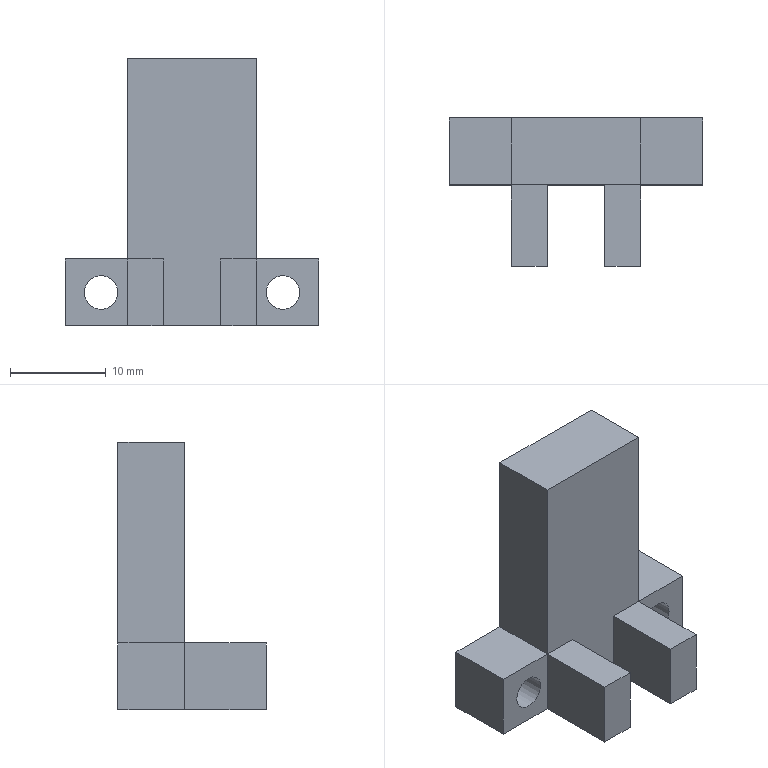Part | NX | 1 solid | 22 faces | box 26.5 x 15.5 x 28 mm | volume 3595 mm3 | plane 20 | cylinder 2 | commonest cylinder face diameters 3.5 x2
STEP:
#1=CARTESIAN_POINT('',(7.75,0.,3.5));
#2=VERTEX_POINT('',#1);
#3=CARTESIAN_POINT('',(9.5,0.,3.5));
#4=DIRECTION('',(0.,-1.,0.));
#5=DIRECTION('',(-1.,0.,0.));
#6=AXIS2_PLACEMENT_3D('',#3,#4,#5);
#7=CIRCLE('',#6,1.75);
#8=EDGE_CURVE('',#2,#2,#7,.T.);
#9=ORIENTED_EDGE('',*,*,#8,.F.);
#10=EDGE_LOOP('',(#9));
#11=FACE_BOUND('',#10,.T.);
#12=CARTESIAN_POINT('',(13.25,0.,7.));
#13=VERTEX_POINT('',#12);
#14=CARTESIAN_POINT('',(13.25,0.,0.));
#15=VERTEX_POINT('',#14);
#16=CARTESIAN_POINT('',(13.25,0.,28.));
#17=DIRECTION('',(0.,0.,-1.));
#18=VECTOR('',#17,1000.);
#19=LINE('',#16,#18);
#20=EDGE_CURVE('',#13,#15,#19,.T.);
#21=ORIENTED_EDGE('',*,*,#20,.F.);
#22=CARTESIAN_POINT('',(6.75,0.,7.));
#23=VERTEX_POINT('',#22);
#24=CARTESIAN_POINT('',(13.25,0.,7.));
#25=DIRECTION('',(1.,0.,0.));
#26=VECTOR('',#25,1000.);
#27=LINE('',#24,#26);
#28=EDGE_CURVE('',#23,#13,#27,.T.);
#29=ORIENTED_EDGE('',*,*,#28,.F.);
#30=CARTESIAN_POINT('',(6.75,0.,0.));
#31=VERTEX_POINT('',#30);
#32=CARTESIAN_POINT('',(6.75,0.,28.));
#33=DIRECTION('',(0.,0.,-1.));
#34=VECTOR('',#33,1000.);
#35=LINE('',#32,#34);
#36=EDGE_CURVE('',#23,#31,#35,.T.);
#37=ORIENTED_EDGE('',*,*,#36,.T.);
#38=CARTESIAN_POINT('',(13.25,0.,0.));
#39=DIRECTION('',(1.,0.,0.));
#40=VECTOR('',#39,1000.);
#41=LINE('',#38,#40);
#42=EDGE_CURVE('',#31,#15,#41,.T.);
#43=ORIENTED_EDGE('',*,*,#42,.T.);
#44=EDGE_LOOP('',(#21,#29,#37,#43));
#45=FACE_BOUND('',#44,.T.);
#46=CARTESIAN_POINT('',(13.25,0.,28.));
#47=DIRECTION('',(0.,1.,0.));
#48=DIRECTION('',(-1.,0.,0.));
#49=AXIS2_PLACEMENT_3D('',#46,#47,#48);
#50=PLANE('',#49);
#51=ADVANCED_FACE('',(#11,#45),#50,.F.);
#52=CARTESIAN_POINT('',(3.,0.,7.));
#53=VERTEX_POINT('',#52);
#54=CARTESIAN_POINT('',(21.25,0.,7.));
#55=DIRECTION('',(-1.,0.,0.));
#56=VECTOR('',#55,1000.);
#57=LINE('',#54,#56);
#58=EDGE_CURVE('',#23,#53,#57,.T.);
#59=ORIENTED_EDGE('',*,*,#58,.F.);
#60=CARTESIAN_POINT('',(6.75,0.,28.));
#61=VERTEX_POINT('',#60);
#62=CARTESIAN_POINT('',(6.75,0.,28.));
#63=DIRECTION('',(0.,0.,-1.));
#64=VECTOR('',#63,1000.);
#65=LINE('',#62,#64);
#66=EDGE_CURVE('',#61,#23,#65,.T.);
#67=ORIENTED_EDGE('',*,*,#66,.F.);
#68=CARTESIAN_POINT('',(-6.75,0.,28.));
#69=VERTEX_POINT('',#68);
#70=CARTESIAN_POINT('',(-13.25,0.,28.));
#71=DIRECTION('',(1.,0.,0.));
#72=VECTOR('',#71,1000.);
#73=LINE('',#70,#72);
#74=EDGE_CURVE('',#69,#61,#73,.T.);
#75=ORIENTED_EDGE('',*,*,#74,.F.);
#76=CARTESIAN_POINT('',(-6.75,0.,7.));
#77=VERTEX_POINT('',#76);
#78=CARTESIAN_POINT('',(-6.75,0.,7.));
#79=DIRECTION('',(0.,0.,1.));
#80=VECTOR('',#79,1000.);
#81=LINE('',#78,#80);
#82=EDGE_CURVE('',#77,#69,#81,.T.);
#83=ORIENTED_EDGE('',*,*,#82,.F.);
#84=CARTESIAN_POINT('',(-3.,0.,7.));
#85=VERTEX_POINT('',#84);
#86=CARTESIAN_POINT('',(21.25,0.,7.));
#87=DIRECTION('',(-1.,0.,0.));
#88=VECTOR('',#87,1000.);
#89=LINE('',#86,#88);
#90=EDGE_CURVE('',#85,#77,#89,.T.);
#91=ORIENTED_EDGE('',*,*,#90,.F.);
#92=CARTESIAN_POINT('',(-3.,0.,0.));
#93=VERTEX_POINT('',#92);
#94=CARTESIAN_POINT('',(-3.,0.,28.));
#95=DIRECTION('',(0.,0.,-1.));
#96=VECTOR('',#95,1000.);
#97=LINE('',#94,#96);
#98=EDGE_CURVE('',#85,#93,#97,.T.);
#99=ORIENTED_EDGE('',*,*,#98,.T.);
#100=CARTESIAN_POINT('',(3.,0.,0.));
#101=VERTEX_POINT('',#100);
#102=CARTESIAN_POINT('',(-3.,0.,0.));
#103=DIRECTION('',(1.,0.,0.));
#104=VECTOR('',#103,1000.);
#105=LINE('',#102,#104);
#106=EDGE_CURVE('',#93,#101,#105,.T.);
#107=ORIENTED_EDGE('',*,*,#106,.T.);
#108=CARTESIAN_POINT('',(3.,0.,28.));
#109=DIRECTION('',(0.,0.,-1.));
#110=VECTOR('',#109,1000.);
#111=LINE('',#108,#110);
#112=EDGE_CURVE('',#53,#101,#111,.T.);
#113=ORIENTED_EDGE('',*,*,#112,.F.);
#114=EDGE_LOOP('',(#59,#67,#75,#83,#91,#99,#107,#113));
#115=FACE_BOUND('',#114,.T.);
#116=CARTESIAN_POINT('',(13.25,0.,28.));
#117=DIRECTION('',(0.,1.,0.));
#118=DIRECTION('',(-1.,0.,0.));
#119=AXIS2_PLACEMENT_3D('',#116,#117,#118);
#120=PLANE('',#119);
#121=ADVANCED_FACE('',(#115),#120,.F.);
#122=CARTESIAN_POINT('',(13.25,7.,7.));
#123=VERTEX_POINT('',#122);
#124=CARTESIAN_POINT('',(13.25,7.,0.));
#125=VERTEX_POINT('',#124);
#126=CARTESIAN_POINT('',(13.25,7.,28.));
#127=DIRECTION('',(0.,0.,-1.));
#128=VECTOR('',#127,1000.);
#129=LINE('',#126,#128);
#130=EDGE_CURVE('',#123,#125,#129,.T.);
#131=ORIENTED_EDGE('',*,*,#130,.F.);
#132=CARTESIAN_POINT('',(13.25,28.,7.));
#133=DIRECTION('',(0.,-1.,0.));
#134=VECTOR('',#133,1000.);
#135=LINE('',#132,#134);
#136=EDGE_CURVE('',#123,#13,#135,.T.);
#137=ORIENTED_EDGE('',*,*,#136,.T.);
#138=ORIENTED_EDGE('',*,*,#20,.T.);
#139=CARTESIAN_POINT('',(13.25,7.,0.));
#140=DIRECTION('',(0.,1.,0.));
#141=VECTOR('',#140,1000.);
#142=LINE('',#139,#141);
#143=EDGE_CURVE('',#15,#125,#142,.T.);
#144=ORIENTED_EDGE('',*,*,#143,.T.);
#145=EDGE_LOOP('',(#131,#137,#138,#144));
#146=FACE_BOUND('',#145,.T.);
#147=CARTESIAN_POINT('',(13.25,7.,28.));
#148=DIRECTION('',(-1.,0.,0.));
#149=DIRECTION('',(0.,0.,1.));
#150=AXIS2_PLACEMENT_3D('',#147,#148,#149);
#151=PLANE('',#150);
#152=ADVANCED_FACE('',(#146),#151,.F.);
#153=CARTESIAN_POINT('',(11.25,7.,3.5));
#154=VERTEX_POINT('',#153);
#155=CARTESIAN_POINT('',(9.5,7.,3.5));
#156=DIRECTION('',(0.,-1.,0.));
#157=DIRECTION('',(1.,0.,0.));
#158=AXIS2_PLACEMENT_3D('',#155,#156,#157);
#159=CIRCLE('',#158,1.75);
#160=EDGE_CURVE('',#154,#154,#159,.T.);
#161=ORIENTED_EDGE('',*,*,#160,.T.);
#162=EDGE_LOOP('',(#161));
#163=FACE_BOUND('',#162,.T.);
#164=CARTESIAN_POINT('',(-7.75,7.,3.5));
#165=VERTEX_POINT('',#164);
#166=CARTESIAN_POINT('',(-9.5,7.,3.5));
#167=DIRECTION('',(0.,-1.,0.));
#168=DIRECTION('',(1.,0.,0.));
#169=AXIS2_PLACEMENT_3D('',#166,#167,#168);
#170=CIRCLE('',#169,1.75);
#171=EDGE_CURVE('',#165,#165,#170,.T.);
#172=ORIENTED_EDGE('',*,*,#171,.T.);
#173=EDGE_LOOP('',(#172));
#174=FACE_BOUND('',#173,.T.);
#175=CARTESIAN_POINT('',(6.75,7.,28.));
#176=VERTEX_POINT('',#175);
#177=CARTESIAN_POINT('',(6.75,7.,7.));
#178=VERTEX_POINT('',#177);
#179=CARTESIAN_POINT('',(6.75,7.,28.));
#180=DIRECTION('',(0.,0.,-1.));
#181=VECTOR('',#180,1000.);
#182=LINE('',#179,#181);
#183=EDGE_CURVE('',#176,#178,#182,.T.);
#184=ORIENTED_EDGE('',*,*,#183,.T.);
#185=CARTESIAN_POINT('',(-13.25,7.,7.));
#186=DIRECTION('',(1.,0.,0.));
#187=VECTOR('',#186,1000.);
#188=LINE('',#185,#187);
#189=EDGE_CURVE('',#178,#123,#188,.T.);
#190=ORIENTED_EDGE('',*,*,#189,.T.);
#191=ORIENTED_EDGE('',*,*,#130,.T.);
#192=CARTESIAN_POINT('',(-13.25,7.,0.));
#193=VERTEX_POINT('',#192);
#194=CARTESIAN_POINT('',(-13.25,7.,0.));
#195=DIRECTION('',(-1.,0.,0.));
#196=VECTOR('',#195,1000.);
#197=LINE('',#194,#196);
#198=EDGE_CURVE('',#125,#193,#197,.T.);
#199=ORIENTED_EDGE('',*,*,#198,.T.);
#200=CARTESIAN_POINT('',(-13.25,7.,7.));
#201=VERTEX_POINT('',#200);
#202=CARTESIAN_POINT('',(-13.25,7.,28.));
#203=DIRECTION('',(0.,0.,-1.));
#204=VECTOR('',#203,1000.);
#205=LINE('',#202,#204);
#206=EDGE_CURVE('',#201,#193,#205,.T.);
#207=ORIENTED_EDGE('',*,*,#206,.F.);
#208=CARTESIAN_POINT('',(-6.75,7.,7.));
#209=VERTEX_POINT('',#208);
#210=CARTESIAN_POINT('',(-13.25,7.,7.));
#211=DIRECTION('',(1.,0.,0.));
#212=VECTOR('',#211,1000.);
#213=LINE('',#210,#212);
#214=EDGE_CURVE('',#201,#209,#213,.T.);
#215=ORIENTED_EDGE('',*,*,#214,.T.);
#216=CARTESIAN_POINT('',(-6.75,7.,28.));
#217=VERTEX_POINT('',#216);
#218=CARTESIAN_POINT('',(-6.75,7.,28.));
#219=DIRECTION('',(0.,0.,1.));
#220=VECTOR('',#219,1000.);
#221=LINE('',#218,#220);
#222=EDGE_CURVE('',#209,#217,#221,.T.);
#223=ORIENTED_EDGE('',*,*,#222,.T.);
#224=CARTESIAN_POINT('',(-13.25,7.,28.));
#225=DIRECTION('',(-1.,0.,0.));
#226=VECTOR('',#225,1000.);
#227=LINE('',#224,#226);
#228=EDGE_CURVE('',#176,#217,#227,.T.);
#229=ORIENTED_EDGE('',*,*,#228,.F.);
#230=EDGE_LOOP('',(#184,#190,#191,#199,#207,#215,#223,#229));
#231=FACE_BOUND('',#230,.T.);
#232=CARTESIAN_POINT('',(-13.25,7.,28.));
#233=DIRECTION('',(0.,-1.,0.));
#234=DIRECTION('',(1.,0.,0.));
#235=AXIS2_PLACEMENT_3D('',#232,#233,#234);
#236=PLANE('',#235);
#237=ADVANCED_FACE('',(#163,#174,#231),#236,.F.);
#238=CARTESIAN_POINT('',(-13.25,0.,7.));
#239=VERTEX_POINT('',#238);
#240=CARTESIAN_POINT('',(-13.25,0.,0.));
#241=VERTEX_POINT('',#240);
#242=CARTESIAN_POINT('',(-13.25,0.,28.));
#243=DIRECTION('',(0.,0.,-1.));
#244=VECTOR('',#243,1000.);
#245=LINE('',#242,#244);
#246=EDGE_CURVE('',#239,#241,#245,.T.);
#247=ORIENTED_EDGE('',*,*,#246,.F.);
#248=CARTESIAN_POINT('',(-13.25,28.,7.));
#249=DIRECTION('',(0.,-1.,0.));
#250=VECTOR('',#249,1000.);
#251=LINE('',#248,#250);
#252=EDGE_CURVE('',#201,#239,#251,.T.);
#253=ORIENTED_EDGE('',*,*,#252,.F.);
#254=ORIENTED_EDGE('',*,*,#206,.T.);
#255=CARTESIAN_POINT('',(-13.25,7.,0.));
#256=DIRECTION('',(0.,-1.,0.));
#257=VECTOR('',#256,1000.);
#258=LINE('',#255,#257);
#259=EDGE_CURVE('',#193,#241,#258,.T.);
#260=ORIENTED_EDGE('',*,*,#259,.T.);
#261=EDGE_LOOP('',(#247,#253,#254,#260));
#262=FACE_BOUND('',#261,.T.);
#263=CARTESIAN_POINT('',(-13.25,7.,28.));
#264=DIRECTION('',(1.,0.,0.));
#265=DIRECTION('',(0.,0.,-1.));
#266=AXIS2_PLACEMENT_3D('',#263,#264,#265);
#267=PLANE('',#266);
#268=ADVANCED_FACE('',(#262),#267,.F.);
#269=CARTESIAN_POINT('',(-6.75,-8.5,7.));
#270=VERTEX_POINT('',#269);
#271=CARTESIAN_POINT('',(-6.75,-8.5,0.));
#272=VERTEX_POINT('',#271);
#273=CARTESIAN_POINT('',(-6.75,-8.5,28.));
#274=DIRECTION('',(0.,0.,-1.));
#275=VECTOR('',#274,1000.);
#276=LINE('',#273,#275);
#277=EDGE_CURVE('',#270,#272,#276,.T.);
#278=ORIENTED_EDGE('',*,*,#277,.F.);
#279=CARTESIAN_POINT('',(-6.75,-8.5,7.));
#280=DIRECTION('',(0.,-1.,0.));
#281=VECTOR('',#280,1000.);
#282=LINE('',#279,#281);
#283=EDGE_CURVE('',#77,#270,#282,.T.);
#284=ORIENTED_EDGE('',*,*,#283,.F.);
#285=CARTESIAN_POINT('',(-6.75,0.,0.));
#286=VERTEX_POINT('',#285);
#287=CARTESIAN_POINT('',(-6.75,0.,28.));
#288=DIRECTION('',(0.,0.,-1.));
#289=VECTOR('',#288,1000.);
#290=LINE('',#287,#289);
#291=EDGE_CURVE('',#77,#286,#290,.T.);
#292=ORIENTED_EDGE('',*,*,#291,.T.);
#293=CARTESIAN_POINT('',(-6.75,0.,0.));
#294=DIRECTION('',(0.,-1.,0.));
#295=VECTOR('',#294,1000.);
#296=LINE('',#293,#295);
#297=EDGE_CURVE('',#286,#272,#296,.T.);
#298=ORIENTED_EDGE('',*,*,#297,.T.);
#299=EDGE_LOOP('',(#278,#284,#292,#298));
#300=FACE_BOUND('',#299,.T.);
#301=CARTESIAN_POINT('',(-6.75,0.,28.));
#302=DIRECTION('',(1.,0.,0.));
#303=DIRECTION('',(0.,1.,0.));
#304=AXIS2_PLACEMENT_3D('',#301,#302,#303);
#305=PLANE('',#304);
#306=ADVANCED_FACE('',(#300),#305,.F.);
#307=CARTESIAN_POINT('',(-3.,-8.5,7.));
#308=VERTEX_POINT('',#307);
#309=CARTESIAN_POINT('',(-3.,-8.5,0.));
#310=VERTEX_POINT('',#309);
#311=CARTESIAN_POINT('',(-3.,-8.5,28.));
#312=DIRECTION('',(0.,0.,-1.));
#313=VECTOR('',#312,1000.);
#314=LINE('',#311,#313);
#315=EDGE_CURVE('',#308,#310,#314,.T.);
#316=ORIENTED_EDGE('',*,*,#315,.F.);
#317=CARTESIAN_POINT('',(21.25,-8.5,7.));
#318=DIRECTION('',(-1.,0.,0.));
#319=VECTOR('',#318,1000.);
#320=LINE('',#317,#319);
#321=EDGE_CURVE('',#308,#270,#320,.T.);
#322=ORIENTED_EDGE('',*,*,#321,.T.);
#323=ORIENTED_EDGE('',*,*,#277,.T.);
#324=CARTESIAN_POINT('',(-6.75,-8.5,0.));
#325=DIRECTION('',(1.,0.,0.));
#326=VECTOR('',#325,1000.);
#327=LINE('',#324,#326);
#328=EDGE_CURVE('',#272,#310,#327,.T.);
#329=ORIENTED_EDGE('',*,*,#328,.T.);
#330=EDGE_LOOP('',(#316,#322,#323,#329));
#331=FACE_BOUND('',#330,.T.);
#332=CARTESIAN_POINT('',(-6.75,-8.5,28.));
#333=DIRECTION('',(0.,1.,0.));
#334=DIRECTION('',(0.,0.,1.));
#335=AXIS2_PLACEMENT_3D('',#332,#333,#334);
#336=PLANE('',#335);
#337=ADVANCED_FACE('',(#331),#336,.F.);
#338=ORIENTED_EDGE('',*,*,#98,.F.);
#339=CARTESIAN_POINT('',(-3.,-8.5,7.));
#340=DIRECTION('',(0.,-1.,0.));
#341=VECTOR('',#340,1000.);
#342=LINE('',#339,#341);
#343=EDGE_CURVE('',#85,#308,#342,.T.);
#344=ORIENTED_EDGE('',*,*,#343,.T.);
#345=ORIENTED_EDGE('',*,*,#315,.T.);
#346=CARTESIAN_POINT('',(-3.,-8.5,0.));
#347=DIRECTION('',(0.,1.,0.));
#348=VECTOR('',#347,1000.);
#349=LINE('',#346,#348);
#350=EDGE_CURVE('',#310,#93,#349,.T.);
#351=ORIENTED_EDGE('',*,*,#350,.T.);
#352=EDGE_LOOP('',(#338,#344,#345,#351));
#353=FACE_BOUND('',#352,.T.);
#354=CARTESIAN_POINT('',(-3.,-8.5,28.));
#355=DIRECTION('',(-1.,0.,0.));
#356=DIRECTION('',(0.,-1.,0.));
#357=AXIS2_PLACEMENT_3D('',#354,#355,#356);
#358=PLANE('',#357);
#359=ADVANCED_FACE('',(#353),#358,.F.);
#360=CARTESIAN_POINT('',(3.,-8.5,7.));
#361=VERTEX_POINT('',#360);
#362=CARTESIAN_POINT('',(3.,-8.5,0.));
#363=VERTEX_POINT('',#362);
#364=CARTESIAN_POINT('',(3.,-8.5,28.));
#365=DIRECTION('',(0.,0.,-1.));
#366=VECTOR('',#365,1000.);
#367=LINE('',#364,#366);
#368=EDGE_CURVE('',#361,#363,#367,.T.);
#369=ORIENTED_EDGE('',*,*,#368,.F.);
#370=CARTESIAN_POINT('',(3.,-8.5,7.));
#371=DIRECTION('',(0.,1.,0.));
#372=VECTOR('',#371,1000.);
#373=LINE('',#370,#372);
#374=EDGE_CURVE('',#361,#53,#373,.T.);
#375=ORIENTED_EDGE('',*,*,#374,.T.);
#376=ORIENTED_EDGE('',*,*,#112,.T.);
#377=CARTESIAN_POINT('',(3.,-8.5,0.));
#378=DIRECTION('',(0.,-1.,0.));
#379=VECTOR('',#378,1000.);
#380=LINE('',#377,#379);
#381=EDGE_CURVE('',#101,#363,#380,.T.);
#382=ORIENTED_EDGE('',*,*,#381,.T.);
#383=EDGE_LOOP('',(#369,#375,#376,#382));
#384=FACE_BOUND('',#383,.T.);
#385=CARTESIAN_POINT('',(3.,-8.5,28.));
#386=DIRECTION('',(1.,0.,0.));
#387=DIRECTION('',(0.,1.,0.));
#388=AXIS2_PLACEMENT_3D('',#385,#386,#387);
#389=PLANE('',#388);
#390=ADVANCED_FACE('',(#384),#389,.F.);
#391=CARTESIAN_POINT('',(6.75,-8.5,7.));
#392=VERTEX_POINT('',#391);
#393=CARTESIAN_POINT('',(6.75,-8.5,0.));
#394=VERTEX_POINT('',#393);
#395=CARTESIAN_POINT('',(6.75,-8.5,28.));
#396=DIRECTION('',(0.,0.,-1.));
#397=VECTOR('',#396,1000.);
#398=LINE('',#395,#397);
#399=EDGE_CURVE('',#392,#394,#398,.T.);
#400=ORIENTED_EDGE('',*,*,#399,.F.);
#401=CARTESIAN_POINT('',(21.25,-8.5,7.));
#402=DIRECTION('',(-1.,0.,0.));
#403=VECTOR('',#402,1000.);
#404=LINE('',#401,#403);
#405=EDGE_CURVE('',#392,#361,#404,.T.);
#406=ORIENTED_EDGE('',*,*,#405,.T.);
#407=ORIENTED_EDGE('',*,*,#368,.T.);
#408=CARTESIAN_POINT('',(6.75,-8.5,0.));
#409=DIRECTION('',(1.,0.,0.));
#410=VECTOR('',#409,1000.);
#411=LINE('',#408,#410);
#412=EDGE_CURVE('',#363,#394,#411,.T.);
#413=ORIENTED_EDGE('',*,*,#412,.T.);
#414=EDGE_LOOP('',(#400,#406,#407,#413));
#415=FACE_BOUND('',#414,.T.);
#416=CARTESIAN_POINT('',(6.75,-8.5,28.));
#417=DIRECTION('',(0.,1.,0.));
#418=DIRECTION('',(-1.,0.,0.));
#419=AXIS2_PLACEMENT_3D('',#416,#417,#418);
#420=PLANE('',#419);
#421=ADVANCED_FACE('',(#415),#420,.F.);
#422=ORIENTED_EDGE('',*,*,#36,.F.);
#423=CARTESIAN_POINT('',(6.75,0.,7.));
#424=DIRECTION('',(0.,-1.,0.));
#425=VECTOR('',#424,1000.);
#426=LINE('',#423,#425);
#427=EDGE_CURVE('',#23,#392,#426,.T.);
#428=ORIENTED_EDGE('',*,*,#427,.T.);
#429=ORIENTED_EDGE('',*,*,#399,.T.);
#430=CARTESIAN_POINT('',(6.75,0.,0.));
#431=DIRECTION('',(0.,1.,0.));
#432=VECTOR('',#431,1000.);
#433=LINE('',#430,#432);
#434=EDGE_CURVE('',#394,#31,#433,.T.);
#435=ORIENTED_EDGE('',*,*,#434,.T.);
#436=EDGE_LOOP('',(#422,#428,#429,#435));
#437=FACE_BOUND('',#436,.T.);
#438=CARTESIAN_POINT('',(6.75,0.,28.));
#439=DIRECTION('',(-1.,0.,0.));
#440=DIRECTION('',(0.,-1.,0.));
#441=AXIS2_PLACEMENT_3D('',#438,#439,#440);
#442=PLANE('',#441);
#443=ADVANCED_FACE('',(#437),#442,.F.);
#444=CARTESIAN_POINT('',(-7.75,0.,3.5));
#445=VERTEX_POINT('',#444);
#446=CARTESIAN_POINT('',(-9.5,0.,3.5));
#447=DIRECTION('',(0.,-1.,0.));
#448=DIRECTION('',(1.,0.,0.));
#449=AXIS2_PLACEMENT_3D('',#446,#447,#448);
#450=CIRCLE('',#449,1.75);
#451=EDGE_CURVE('',#445,#445,#450,.T.);
#452=ORIENTED_EDGE('',*,*,#451,.F.);
#453=EDGE_LOOP('',(#452));
#454=FACE_BOUND('',#453,.T.);
#455=ORIENTED_EDGE('',*,*,#291,.F.);
#456=CARTESIAN_POINT('',(-6.75,0.,7.));
#457=DIRECTION('',(1.,0.,0.));
#458=VECTOR('',#457,1000.);
#459=LINE('',#456,#458);
#460=EDGE_CURVE('',#239,#77,#459,.T.);
#461=ORIENTED_EDGE('',*,*,#460,.F.);
#462=ORIENTED_EDGE('',*,*,#246,.T.);
#463=CARTESIAN_POINT('',(-13.25,0.,0.));
#464=DIRECTION('',(1.,0.,0.));
#465=VECTOR('',#464,1000.);
#466=LINE('',#463,#465);
#467=EDGE_CURVE('',#241,#286,#466,.T.);
#468=ORIENTED_EDGE('',*,*,#467,.T.);
#469=EDGE_LOOP('',(#455,#461,#462,#468));
#470=FACE_BOUND('',#469,.T.);
#471=CARTESIAN_POINT('',(13.25,0.,28.));
#472=DIRECTION('',(0.,1.,0.));
#473=DIRECTION('',(-1.,0.,0.));
#474=AXIS2_PLACEMENT_3D('',#471,#472,#473);
#475=PLANE('',#474);
#476=ADVANCED_FACE('',(#454,#470),#475,.F.);
#477=ORIENTED_EDGE('',*,*,#74,.T.);
#478=CARTESIAN_POINT('',(6.75,0.,28.));
#479=DIRECTION('',(0.,1.,0.));
#480=VECTOR('',#479,1000.);
#481=LINE('',#478,#480);
#482=EDGE_CURVE('',#61,#176,#481,.T.);
#483=ORIENTED_EDGE('',*,*,#482,.T.);
#484=ORIENTED_EDGE('',*,*,#228,.T.);
#485=CARTESIAN_POINT('',(-6.75,0.,28.));
#486=DIRECTION('',(0.,-1.,0.));
#487=VECTOR('',#486,1000.);
#488=LINE('',#485,#487);
#489=EDGE_CURVE('',#217,#69,#488,.T.);
#490=ORIENTED_EDGE('',*,*,#489,.T.);
#491=EDGE_LOOP('',(#477,#483,#484,#490));
#492=FACE_BOUND('',#491,.T.);
#493=CARTESIAN_POINT('',(0.,0.,28.));
#494=DIRECTION('',(0.,0.,-1.));
#495=DIRECTION('',(-1.,0.,0.));
#496=AXIS2_PLACEMENT_3D('',#493,#494,#495);
#497=PLANE('',#496);
#498=ADVANCED_FACE('',(#492),#497,.F.);
#499=ORIENTED_EDGE('',*,*,#143,.F.);
#500=ORIENTED_EDGE('',*,*,#42,.F.);
#501=ORIENTED_EDGE('',*,*,#434,.F.);
#502=ORIENTED_EDGE('',*,*,#412,.F.);
#503=ORIENTED_EDGE('',*,*,#381,.F.);
#504=ORIENTED_EDGE('',*,*,#106,.F.);
#505=ORIENTED_EDGE('',*,*,#350,.F.);
#506=ORIENTED_EDGE('',*,*,#328,.F.);
#507=ORIENTED_EDGE('',*,*,#297,.F.);
#508=ORIENTED_EDGE('',*,*,#467,.F.);
#509=ORIENTED_EDGE('',*,*,#259,.F.);
#510=ORIENTED_EDGE('',*,*,#198,.F.);
#511=EDGE_LOOP('',(#499,#500,#501,#502,#503,#504,#505,#506,#507,#508,#509,#510));
#512=FACE_BOUND('',#511,.T.);
#513=CARTESIAN_POINT('',(0.,0.,0.));
#514=DIRECTION('',(0.,0.,-1.));
#515=DIRECTION('',(-1.,0.,0.));
#516=AXIS2_PLACEMENT_3D('',#513,#514,#515);
#517=PLANE('',#516);
#518=ADVANCED_FACE('',(#512),#517,.T.);
#519=ORIENTED_EDGE('',*,*,#405,.F.);
#520=ORIENTED_EDGE('',*,*,#427,.F.);
#521=ORIENTED_EDGE('',*,*,#58,.T.);
#522=ORIENTED_EDGE('',*,*,#374,.F.);
#523=EDGE_LOOP('',(#519,#520,#521,#522));
#524=FACE_BOUND('',#523,.T.);
#525=CARTESIAN_POINT('',(21.25,-8.5,7.));
#526=DIRECTION('',(0.,0.,-1.));
#527=DIRECTION('',(-1.,0.,0.));
#528=AXIS2_PLACEMENT_3D('',#525,#526,#527);
#529=PLANE('',#528);
#530=ADVANCED_FACE('',(#524),#529,.F.);
#531=ORIENTED_EDGE('',*,*,#90,.T.);
#532=ORIENTED_EDGE('',*,*,#283,.T.);
#533=ORIENTED_EDGE('',*,*,#321,.F.);
#534=ORIENTED_EDGE('',*,*,#343,.F.);
#535=EDGE_LOOP('',(#531,#532,#533,#534));
#536=FACE_BOUND('',#535,.T.);
#537=CARTESIAN_POINT('',(21.25,-8.5,7.));
#538=DIRECTION('',(0.,0.,-1.));
#539=DIRECTION('',(-1.,0.,0.));
#540=AXIS2_PLACEMENT_3D('',#537,#538,#539);
#541=PLANE('',#540);
#542=ADVANCED_FACE('',(#536),#541,.F.);
#543=ORIENTED_EDGE('',*,*,#252,.T.);
#544=ORIENTED_EDGE('',*,*,#460,.T.);
#545=CARTESIAN_POINT('',(-6.75,28.,7.));
#546=DIRECTION('',(0.,-1.,0.));
#547=VECTOR('',#546,1000.);
#548=LINE('',#545,#547);
#549=EDGE_CURVE('',#209,#77,#548,.T.);
#550=ORIENTED_EDGE('',*,*,#549,.F.);
#551=ORIENTED_EDGE('',*,*,#214,.F.);
#552=EDGE_LOOP('',(#543,#544,#550,#551));
#553=FACE_BOUND('',#552,.T.);
#554=CARTESIAN_POINT('',(-6.75,28.,7.));
#555=DIRECTION('',(0.,0.,-1.));
#556=DIRECTION('',(-1.,0.,0.));
#557=AXIS2_PLACEMENT_3D('',#554,#555,#556);
#558=PLANE('',#557);
#559=ADVANCED_FACE('',(#553),#558,.F.);
#560=ORIENTED_EDGE('',*,*,#549,.T.);
#561=ORIENTED_EDGE('',*,*,#82,.T.);
#562=ORIENTED_EDGE('',*,*,#489,.F.);
#563=ORIENTED_EDGE('',*,*,#222,.F.);
#564=EDGE_LOOP('',(#560,#561,#562,#563));
#565=FACE_BOUND('',#564,.T.);
#566=CARTESIAN_POINT('',(-6.75,28.,7.));
#567=DIRECTION('',(1.,0.,0.));
#568=DIRECTION('',(0.,1.,0.));
#569=AXIS2_PLACEMENT_3D('',#566,#567,#568);
#570=PLANE('',#569);
#571=ADVANCED_FACE('',(#565),#570,.F.);
#572=CARTESIAN_POINT('',(6.75,28.,7.));
#573=DIRECTION('',(0.,-1.,0.));
#574=VECTOR('',#573,1000.);
#575=LINE('',#572,#574);
#576=EDGE_CURVE('',#178,#23,#575,.T.);
#577=ORIENTED_EDGE('',*,*,#576,.T.);
#578=ORIENTED_EDGE('',*,*,#28,.T.);
#579=ORIENTED_EDGE('',*,*,#136,.F.);
#580=ORIENTED_EDGE('',*,*,#189,.F.);
#581=EDGE_LOOP('',(#577,#578,#579,#580));
#582=FACE_BOUND('',#581,.T.);
#583=CARTESIAN_POINT('',(13.25,28.,7.));
#584=DIRECTION('',(0.,0.,-1.));
#585=DIRECTION('',(-1.,0.,0.));
#586=AXIS2_PLACEMENT_3D('',#583,#584,#585);
#587=PLANE('',#586);
#588=ADVANCED_FACE('',(#582),#587,.F.);
#589=ORIENTED_EDGE('',*,*,#482,.F.);
#590=ORIENTED_EDGE('',*,*,#66,.T.);
#591=ORIENTED_EDGE('',*,*,#576,.F.);
#592=ORIENTED_EDGE('',*,*,#183,.F.);
#593=EDGE_LOOP('',(#589,#590,#591,#592));
#594=FACE_BOUND('',#593,.T.);
#595=CARTESIAN_POINT('',(6.75,28.,28.));
#596=DIRECTION('',(-1.,0.,0.));
#597=DIRECTION('',(0.,-1.,0.));
#598=AXIS2_PLACEMENT_3D('',#595,#596,#597);
#599=PLANE('',#598);
#600=ADVANCED_FACE('',(#594),#599,.F.);
#601=ORIENTED_EDGE('',*,*,#451,.T.);
#602=EDGE_LOOP('',(#601));
#603=FACE_BOUND('',#602,.T.);
#604=ORIENTED_EDGE('',*,*,#171,.F.);
#605=EDGE_LOOP('',(#604));
#606=FACE_BOUND('',#605,.T.);
#607=CARTESIAN_POINT('',(-9.5,28.,3.5));
#608=DIRECTION('',(0.,-1.,0.));
#609=DIRECTION('',(1.,0.,0.));
#610=AXIS2_PLACEMENT_3D('',#607,#608,#609);
#611=CYLINDRICAL_SURFACE('',#610,1.75);
#612=ADVANCED_FACE('',(#603,#606),#611,.F.);
#613=ORIENTED_EDGE('',*,*,#8,.T.);
#614=EDGE_LOOP('',(#613));
#615=FACE_BOUND('',#614,.T.);
#616=ORIENTED_EDGE('',*,*,#160,.F.);
#617=EDGE_LOOP('',(#616));
#618=FACE_BOUND('',#617,.T.);
#619=CARTESIAN_POINT('',(9.5,28.,3.5));
#620=DIRECTION('',(0.,-1.,0.));
#621=DIRECTION('',(1.,0.,0.));
#622=AXIS2_PLACEMENT_3D('',#619,#620,#621);
#623=CYLINDRICAL_SURFACE('',#622,1.75);
#624=ADVANCED_FACE('',(#615,#618),#623,.F.);
#625=CLOSED_SHELL('',(#51,#121,#152,#237,#268,#306,#337,#359,#390,#421,#443,#476,#498,#518,#530,#542,#559,#571,#588,#600,#612,#624));
#626=MANIFOLD_SOLID_BREP('',#625);
#627=(LENGTH_UNIT()NAMED_UNIT(*)SI_UNIT(.MILLI.,.METRE.));
#628=UNCERTAINTY_MEASURE_WITH_UNIT(LENGTH_MEASURE(0.00001),#627,'','');
#629=(NAMED_UNIT(*)PLANE_ANGLE_UNIT()SI_UNIT($,.RADIAN.));
#630=(NAMED_UNIT(*)SI_UNIT($,.STERADIAN.)SOLID_ANGLE_UNIT());
#631=(GEOMETRIC_REPRESENTATION_CONTEXT(3)GLOBAL_UNCERTAINTY_ASSIGNED_CONTEXT((#628))GLOBAL_UNIT_ASSIGNED_CONTEXT((#627,#629,#630))REPRESENTATION_CONTEXT('',''));
#632=ADVANCED_BREP_SHAPE_REPRESENTATION('',(#626),#631);